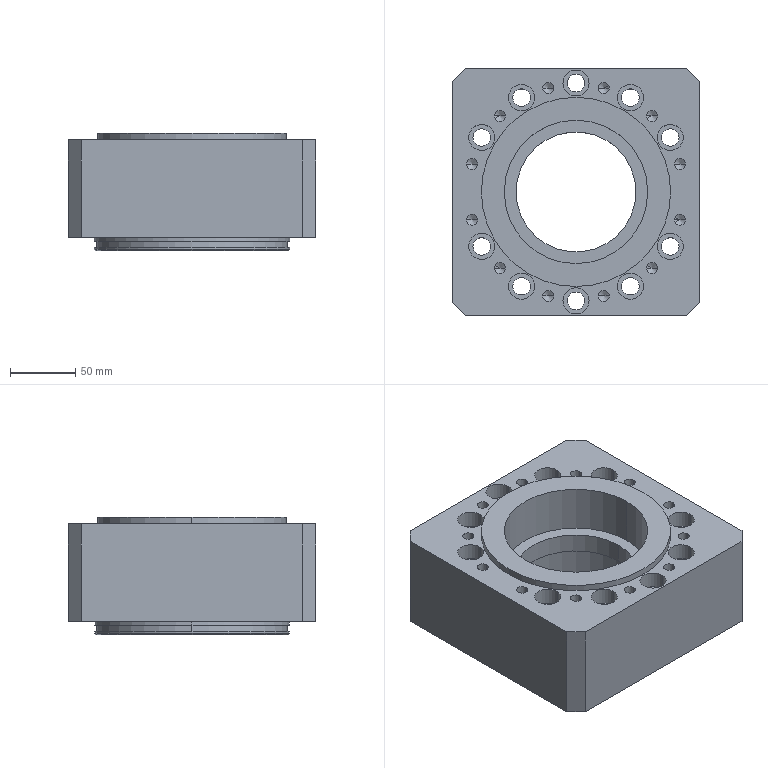Part | SolidWorks | features ICE 14, Chamfer 4, HoleWzd 4, CirPattern 3, Extrusion 1 | 1 solid | 146 faces | box 190 x 190 x 90 mm | volume 1988671 mm3 | cylinder 86 | cone 34 | plane 26 | commonest cylinder face diameters 8.5 x24 13.5 x20 20 x20 5 x8 110 x4 150 x4